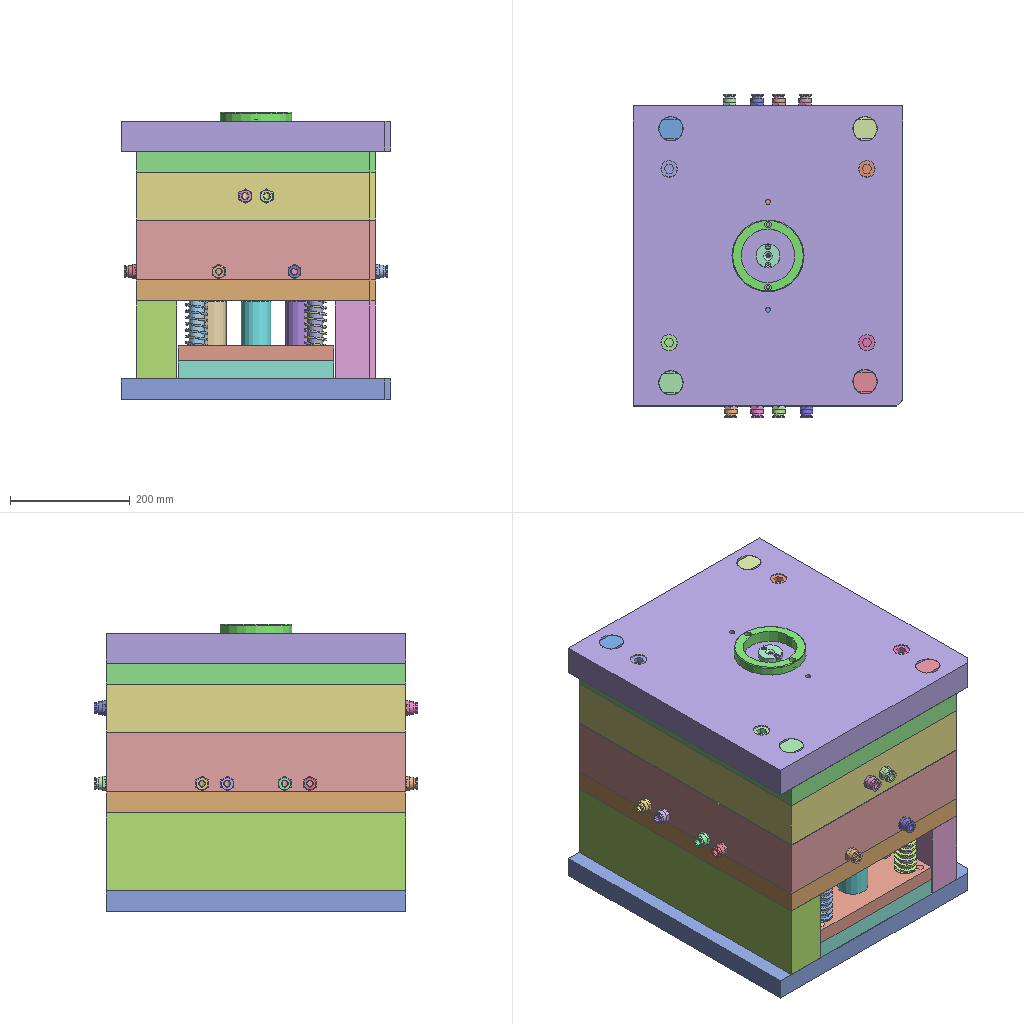Assembly | STEP file | 188 different items | 188 placed | box 450 x 540 x 480 mm
Parts list (item | name | quantity | parent item | size | volume):
1 | 1_id114_xmt_txt | x1 | in SL2-MOLD_xmt_txt | 21 x 31.9 x 24.249 mm | 5376 mm3
2 | 1_id118_xmt_txt | x1 | in SL2-MOLD_xmt_txt | 21 x 31.9 x 24.249 mm | 5376 mm3
3 | 1_id122_xmt_txt | x1 | in SL2-MOLD_xmt_txt | 21 x 31.9 x 24.249 mm | 5376 mm3
4 | 1_id126_xmt_txt | x1 | in SL2-MOLD_xmt_txt | 21 x 31.9 x 24.249 mm | 5376 mm3
5 | 1_id130_xmt_txt | x1 | in SL2-MOLD_xmt_txt | 10 x 10 x 26 mm | 960.822 mm3
6 | 1_id134_xmt_txt | x1 | in SL2-MOLD_xmt_txt | 10 x 10 x 26 mm | 960.822 mm3
7 | 1_id138_xmt_txt | x1 | in SL2-MOLD_xmt_txt | 10 x 10 x 26 mm | 960.822 mm3
8 | 1_id142_xmt_txt | x1 | in SL2-MOLD_xmt_txt | 10 x 10 x 26 mm | 960.822 mm3
9 | 1_id146_xmt_txt | x1 | in SL2-MOLD_xmt_txt | 10 x 10 x 26 mm | 960.822 mm3
10 | 1_id150_xmt_txt | x1 | in SL2-MOLD_xmt_txt | 10 x 10 x 26 mm | 960.822 mm3
11 | 1_id154_xmt_txt | x1 | in SL2-MOLD_xmt_txt | 10 x 10 x 26 mm | 960.822 mm3
12 | 1_id158_xmt_txt | x1 | in SL2-MOLD_xmt_txt | 10 x 10 x 26 mm | 960.822 mm3
13 | 1_id162_xmt_txt | x1 | in SL2-MOLD_xmt_txt | 10 x 10 x 26 mm | 960.822 mm3
14 | 1_id166_xmt_txt | x1 | in SL2-MOLD_xmt_txt | 10 x 10 x 26 mm | 960.822 mm3
15 | 1_id170_xmt_txt | x1 | in SL2-MOLD_xmt_txt | 10 x 10 x 26 mm | 960.822 mm3
16 | 1_id174_xmt_txt | x1 | in SL2-MOLD_xmt_txt | 10 x 10 x 26 mm | 960.822 mm3
17 | 1_id282_xmt_txt | x1 | in SL2-MOLD_xmt_txt | 21 x 31.9 x 24.249 mm | 5376 mm3
18 | 1_id286_xmt_txt | x1 | in SL2-MOLD_xmt_txt | 21 x 31.9 x 24.249 mm | 5376 mm3
19 | 1_id290_xmt_txt | x1 | in SL2-MOLD_xmt_txt | 21 x 31.9 x 24.249 mm | 5376 mm3
20 | 1_id294_xmt_txt | x1 | in SL2-MOLD_xmt_txt | 21 x 31.9 x 24.249 mm | 5376 mm3
21 | 1_id298_xmt_txt | x1 | in SL2-MOLD_xmt_txt | 31.9 x 21 x 24.249 mm | 5376 mm3
22 | 1_id302_xmt_txt | x1 | in SL2-MOLD_xmt_txt | 31.9 x 21 x 24.249 mm | 5376 mm3
23 | 1_id306_xmt_txt | x1 | in SL2-MOLD_xmt_txt | 31.9 x 21 x 24.249 mm | 5376 mm3
24 | 1_id310_xmt_txt | x1 | in SL2-MOLD_xmt_txt | 31.9 x 21 x 24.249 mm | 5376 mm3
25 | 1_id314_xmt_txt | x1 | in SL2-MOLD_xmt_txt | 31.9 x 21 x 24.249 mm | 5376 mm3
26 | 1_id318_xmt_txt | x1 | in SL2-MOLD_xmt_txt | 31.9 x 21 x 24.249 mm | 5376 mm3
27 | 1_id322_xmt_txt | x1 | in SL2-MOLD_xmt_txt | 31.9 x 21 x 24.249 mm | 5376 mm3
28 | 1_id326_xmt_txt | x1 | in SL2-MOLD_xmt_txt | 31.9 x 21 x 24.249 mm | 5376 mm3
29 | 1_id330_xmt_txt | x1 | in SL2-MOLD_xmt_txt | 18 x 18 x 47 mm | 6453 mm3
30 | 1_id334_xmt_txt | x1 | in SL2-MOLD_xmt_txt | 18 x 18 x 47 mm | 6453 mm3
31 | 1_id338_xmt_txt | x1 | in SL2-MOLD_xmt_txt | 18 x 18 x 47 mm | 6453 mm3
32 | 1_id342_xmt_txt | x1 | in SL2-MOLD_xmt_txt | 18 x 18 x 47 mm | 6453 mm3
33 | 1_id346_xmt_txt | x1 | in SL2-MOLD_xmt_txt | 18 x 18 x 47 mm | 6453 mm3
34 | 1_id350_xmt_txt | x1 | in SL2-MOLD_xmt_txt | 18 x 18 x 47 mm | 6453 mm3
35 | 1_id442_xmt_txt | x1 | in SL2-MOLD_xmt_txt | 40 x 40 x 350 mm | 322067 mm3
36 | 1_id446_xmt_txt | x1 | in SL2-MOLD_xmt_txt | 40 x 40 x 350 mm | 322067 mm3
37 | 1_id450_xmt_txt | x1 | in SL2-MOLD_xmt_txt | 40 x 40 x 350 mm | 322067 mm3
38 | 1_id454_xmt_txt | x1 | in SL2-MOLD_xmt_txt | 40 x 40 x 350 mm | 322067 mm3
39 | 1_id458_xmt_txt | x1 | in SL2-MOLD_xmt_txt | 48.005 x 48.005 x 35 mm | 28920 mm3
40 | 1_id462_xmt_txt | x1 | in SL2-MOLD_xmt_txt | 48.005 x 48.005 x 35 mm | 28920 mm3
41 | 1_id466_xmt_txt | x1 | in SL2-MOLD_xmt_txt | 48.005 x 48.005 x 35 mm | 28920 mm3
42 | 1_id470_xmt_txt | x1 | in SL2-MOLD_xmt_txt | 48.005 x 48.005 x 35 mm | 28920 mm3
43 | 1_id474_xmt_txt | x1 | in SL2-MOLD_xmt_txt | 54 x 54 x 80 mm | 71084 mm3
44 | 1_id478_xmt_txt | x1 | in SL2-MOLD_xmt_txt | 54 x 54 x 80 mm | 71084 mm3
45 | 1_id482_xmt_txt | x1 | in SL2-MOLD_xmt_txt | 54 x 54 x 80 mm | 71084 mm3
46 | 1_id486_xmt_txt | x1 | in SL2-MOLD_xmt_txt | 54 x 54 x 80 mm | 71084 mm3
47 | 1_id490_xmt_txt | x1 | in SL2-MOLD_xmt_txt | 54 x 54 x 80 mm | 71084 mm3
48 | 1_id494_xmt_txt | x1 | in SL2-MOLD_xmt_txt | 54 x 54 x 80 mm | 71084 mm3
49 | 1_id498_xmt_txt | x1 | in SL2-MOLD_xmt_txt | 54 x 54 x 80 mm | 71084 mm3
50 | 1_id502_xmt_txt | x1 | in SL2-MOLD_xmt_txt | 54 x 54 x 80 mm | 71084 mm3
51 | 1_id506_xmt_txt | x1 | in SL2-MOLD_xmt_txt | 120 x 120 x 20 mm | 95777 mm3
52 | 1_id530_xmt_txt | x1 | in SL2-MOLD_xmt_txt | 8 x 8 x 63 mm | 1811 mm3
53 | 1_id534_xmt_txt | x1 | in SL2-MOLD_xmt_txt | 8 x 8 x 63 mm | 1811 mm3
54 | 1_id538_xmt_txt | x1 | in SL2-MOLD_xmt_txt | 28 x 28 x 214 mm | 66281 mm3
55 | 1_id542_xmt_txt | x1 | in SL2-MOLD_xmt_txt | 28 x 28 x 214 mm | 66281 mm3
56 | 1_id546_xmt_txt | x1 | in SL2-MOLD_xmt_txt | 28 x 28 x 214 mm | 66281 mm3
57 | 1_id550_xmt_txt | x1 | in SL2-MOLD_xmt_txt | 28 x 28 x 214 mm | 66281 mm3
58 | 1_id554_xmt_txt | x1 | in SL2-MOLD_xmt_txt | 27 x 27 x 96 mm | 22322 mm3
59 | 1_id558_xmt_txt | x1 | in SL2-MOLD_xmt_txt | 27 x 27 x 96 mm | 22322 mm3
60 | 1_id562_xmt_txt | x1 | in SL2-MOLD_xmt_txt | 27 x 27 x 96 mm | 22322 mm3
61 | 1_id566_xmt_txt | x1 | in SL2-MOLD_xmt_txt | 27 x 27 x 96 mm | 22322 mm3
62 | 1_id570_xmt_txt | x1 | in SL2-MOLD_xmt_txt | 20 x 20 x 44 mm | 10770 mm3
63 | 1_id574_xmt_txt | x1 | in SL2-MOLD_xmt_txt | 20 x 20 x 44 mm | 10770 mm3
64 | 1_id578_xmt_txt | x1 | in SL2-MOLD_xmt_txt | 20 x 20 x 44 mm | 10770 mm3
65 | 1_id582_xmt_txt | x1 | in SL2-MOLD_xmt_txt | 20 x 20 x 44 mm | 10770 mm3
66 | 1_id586_xmt_txt | x1 | in SL2-MOLD_xmt_txt | 24 x 24 x 236 mm | 50039 mm3
67 | 1_id58_xmt_txt | x1 | in SL2-MOLD_xmt_txt | 18 x 18 x 47 mm | 6453 mm3
68 | 1_id590_xmt_txt | x1 | in SL2-MOLD_xmt_txt | 24 x 24 x 236 mm | 50039 mm3
69 | 1_id594_xmt_txt | x1 | in SL2-MOLD_xmt_txt | 24 x 24 x 236 mm | 50039 mm3
70 | 1_id598_xmt_txt | x1 | in SL2-MOLD_xmt_txt | 24 x 24 x 236 mm | 50039 mm3
71 | 1_id602_xmt_txt | x1 | in SL2-MOLD_xmt_txt | 24 x 24 x 236 mm | 50039 mm3
72 | 1_id606_xmt_txt | x1 | in SL2-MOLD_xmt_txt | 24 x 24 x 236 mm | 50039 mm3
73 | 1_id610_xmt_txt | x1 | in SL2-MOLD_xmt_txt | 18 x 18 x 55 mm | 7362 mm3
74 | 1_id614_xmt_txt | x1 | in SL2-MOLD_xmt_txt | 18 x 18 x 55 mm | 7362 mm3
75 | 1_id618_xmt_txt | x1 | in SL2-MOLD_xmt_txt | 18 x 18 x 55 mm | 7362 mm3
76 | 1_id622_xmt_txt | x1 | in SL2-MOLD_xmt_txt | 18 x 18 x 55 mm | 7362 mm3
77 | 1_id626_xmt_txt | x1 | in SL2-MOLD_xmt_txt | 18 x 18 x 55 mm | 7362 mm3
78 | 1_id62_xmt_txt | x1 | in SL2-MOLD_xmt_txt | 18 x 18 x 47 mm | 6453 mm3
79 | 1_id630_xmt_txt | x1 | in SL2-MOLD_xmt_txt | 18 x 18 x 55 mm | 7362 mm3
80 | 1_id634_xmt_txt | x1 | in SL2-MOLD_xmt_txt | 30 x 30 x 231 mm | 114179 mm3
81 | 1_id638_xmt_txt | x1 | in SL2-MOLD_xmt_txt | 30 x 30 x 231 mm | 114179 mm3
82 | 1_id642_xmt_txt | x1 | in SL2-MOLD_xmt_txt | 30 x 30 x 231 mm | 114179 mm3
83 | 1_id646_xmt_txt | x1 | in SL2-MOLD_xmt_txt | 30 x 30 x 231 mm | 114179 mm3
84 | 1_id654_xmt_txt | x1 | in SL2-MOLD_xmt_txt | 37 x 37 x 150 mm | 21369 mm3
85 | 1_id658_xmt_txt | x1 | in SL2-MOLD_xmt_txt | 37 x 37 x 150 mm | 21369 mm3
86 | 1_id662_xmt_txt | x1 | in SL2-MOLD_xmt_txt | 37 x 37 x 150 mm | 21369 mm3
87 | 1_id666_xmt_txt | x1 | in SL2-MOLD_xmt_txt | 37 x 37 x 150 mm | 21369 mm3
88 | 1_id66_xmt_txt | x1 | in SL2-MOLD_xmt_txt | 18 x 18 x 47 mm | 6453 mm3
89 | 1_id670_xmt_txt | x1 | in SL2-MOLD_xmt_txt | 28 x 28 x 185 mm | 57057 mm3
90 | 1_id674_xmt_txt | x1 | in SL2-MOLD_xmt_txt | 28 x 28 x 185 mm | 57057 mm3
91 | 1_id678_xmt_txt | x1 | in SL2-MOLD_xmt_txt | 28 x 28 x 185 mm | 57057 mm3
92 | 1_id682_xmt_txt | x1 | in SL2-MOLD_xmt_txt | 28 x 28 x 185 mm | 57057 mm3
93 | 1_id686_xmt_txt | x1 | in SL2-MOLD_xmt_txt | 18 x 18 x 47 mm | 6453 mm3
94 | 1_id690_xmt_txt | x1 | in SL2-MOLD_xmt_txt | 18 x 18 x 47 mm | 6453 mm3
95 | 1_id694_xmt_txt | x1 | in SL2-MOLD_xmt_txt | 18 x 18 x 47 mm | 6453 mm3
96 | 1_id698_xmt_txt | x1 | in SL2-MOLD_xmt_txt | 18 x 18 x 47 mm | 6453 mm3
97 | 1_id706_xmt_txt | x1 | in SL2-MOLD_xmt_txt | 40 x 40 x 95 mm | 34804 mm3
98 | 1_id70_xmt_txt | x1 | in SL2-MOLD_xmt_txt | 18 x 18 x 47 mm | 6453 mm3
99 | 1_id74_xmt_txt | x1 | in SL2-MOLD_xmt_txt | 18 x 18 x 47 mm | 6453 mm3
100 | 1_id78_xmt_txt | x1 | in SL2-MOLD_xmt_txt | 18 x 18 x 47 mm | 6453 mm3
101 | 1_id82_xmt_txt | x1 | in SL2-MOLD_xmt_txt | 18 x 18 x 47 mm | 6453 mm3
102 | 1_id86_xmt_txt | x1 | in SL2-MOLD_xmt_txt | 18 x 18 x 47 mm | 6453 mm3
103 | 2_id514_xmt_txt | x1 | in SL2-MOLD_xmt_txt | 8.5 x 8.5 x 17 mm | 477.285 mm3
104 | 3_id510_xmt_txt | x1 | in SL2-MOLD_xmt_txt | 8.5 x 8.5 x 17 mm | 477.285 mm3
105 | SL2-MOLD_id102_xmt_txt | x1 | in SL2-MOLD_xmt_txt | 50 x 50 x 130 mm | 253722 mm3
106 | SL2-MOLD_id106_xmt_txt | x1 | in SL2-MOLD_xmt_txt | 50 x 50 x 130 mm | 253722 mm3
107 | SL2-MOLD_id10_xmt_txt | x1 | in SL2-MOLD_xmt_txt | 50 x 11.99 x 16.246 mm | 7285 mm3
108 | SL2-MOLD_id110_xmt_txt | x1 | in SL2-MOLD_xmt_txt | 50 x 50 x 130 mm | 253722 mm3
109 | SL2-MOLD_id14_xmt_txt | x1 | in SL2-MOLD_xmt_txt | 45 x 110 x 10 mm | 48642 mm3
110 | SL2-MOLD_id178_xmt_txt | x1 | in SL2-MOLD_xmt_txt | 20 x 20 x 95 mm | 5358 mm3
111 | SL2-MOLD_id182_xmt_txt | x1 | in SL2-MOLD_xmt_txt | 20 x 20 x 95 mm | 5358 mm3
112 | SL2-MOLD_id186_xmt_txt | x1 | in SL2-MOLD_xmt_txt | 20 x 20 x 95 mm | 5358 mm3
113 | SL2-MOLD_id18_xmt_txt | x1 | in SL2-MOLD_xmt_txt | 110 x 40 x 10 mm | 43142 mm3
114 | SL2-MOLD_id190_xmt_txt | x1 | in SL2-MOLD_xmt_txt | 20 x 20 x 95 mm | 5358 mm3
115 | SL2-MOLD_id194_xmt_txt | x1 | in SL2-MOLD_xmt_txt | 20 x 20 x 95 mm | 5358 mm3
116 | SL2-MOLD_id198_xmt_txt | x1 | in SL2-MOLD_xmt_txt | 20 x 20 x 95 mm | 5358 mm3
117 | SL2-MOLD_id202_xmt_txt | x1 | in SL2-MOLD_xmt_txt | 20 x 20 x 95 mm | 5358 mm3
118 | SL2-MOLD_id206_xmt_txt | x1 | in SL2-MOLD_xmt_txt | 20 x 20 x 95 mm | 5358 mm3
119 | SL2-MOLD_id210_xmt_txt | x1 | in SL2-MOLD_xmt_txt | 20 x 20 x 95 mm | 5358 mm3
120 | SL2-MOLD_id214_xmt_txt | x1 | in SL2-MOLD_xmt_txt | 20 x 20 x 95 mm | 5358 mm3
121 | SL2-MOLD_id218_xmt_txt | x1 | in SL2-MOLD_xmt_txt | 20 x 20 x 95 mm | 5358 mm3
122 | SL2-MOLD_id222_xmt_txt | x1 | in SL2-MOLD_xmt_txt | 20 x 20 x 95 mm | 5358 mm3
123 | SL2-MOLD_id226_xmt_txt | x1 | in SL2-MOLD_xmt_txt | 20 x 20 x 95 mm | 5358 mm3
124 | SL2-MOLD_id22_xmt_txt | x1 | in SL2-MOLD_xmt_txt | 110 x 40 x 10 mm | 43142 mm3
125 | SL2-MOLD_id230_xmt_txt | x1 | in SL2-MOLD_xmt_txt | 20 x 20 x 95 mm | 5358 mm3
126 | SL2-MOLD_id234_xmt_txt | x1 | in SL2-MOLD_xmt_txt | 20 x 20 x 95 mm | 5358 mm3
127 | SL2-MOLD_id238_xmt_txt | x1 | in SL2-MOLD_xmt_txt | 20 x 20 x 95 mm | 5358 mm3
128 | SL2-MOLD_id242_xmt_txt | x1 | in SL2-MOLD_xmt_txt | 20 x 20 x 95 mm | 5358 mm3
129 | SL2-MOLD_id246_xmt_txt | x1 | in SL2-MOLD_xmt_txt | 20 x 20 x 95 mm | 5358 mm3
130 | SL2-MOLD_id250_xmt_txt | x1 | in SL2-MOLD_xmt_txt | 20 x 20 x 95 mm | 5358 mm3
131 | SL2-MOLD_id254_xmt_txt | x1 | in SL2-MOLD_xmt_txt | 20 x 20 x 95 mm | 5358 mm3
132 | SL2-MOLD_id258_xmt_txt | x1 | in SL2-MOLD_xmt_txt | 20 x 20 x 95 mm | 5358 mm3
133 | SL2-MOLD_id262_xmt_txt | x1 | in SL2-MOLD_xmt_txt | 20 x 20 x 95 mm | 5358 mm3
134 | SL2-MOLD_id266_xmt_txt | x1 | in SL2-MOLD_xmt_txt | 20 x 20 x 95 mm | 5358 mm3
135 | SL2-MOLD_id26_xmt_txt | x1 | in SL2-MOLD_xmt_txt | 45 x 110 x 10 mm | 48642 mm3
136 | SL2-MOLD_id270_xmt_txt | x1 | in SL2-MOLD_xmt_txt | 20 x 20 x 95 mm | 5358 mm3
137 | SL2-MOLD_id274_xmt_txt | x1 | in SL2-MOLD_xmt_txt | 20 x 20 x 95 mm | 5358 mm3
138 | SL2-MOLD_id278_xmt_txt | x1 | in SL2-MOLD_xmt_txt | 20 x 20 x 95 mm | 5358 mm3
139 | SL2-MOLD_id30_xmt_txt | x1 | in SL2-MOLD_xmt_txt | 11.99 x 50 x 16.246 mm | 7285 mm3
140 | SL2-MOLD_id34_xmt_txt | x1 | in SL2-MOLD_xmt_txt | 11.99 x 50 x 16.246 mm | 7285 mm3
141 | SL2-MOLD_id354_xmt_txt | x1 | in SL2-MOLD_xmt_txt | 265 x 420 x 8 mm | 688291 mm3
142 | SL2-MOLD_id358_xmt_txt | x1 | in SL2-MOLD_xmt_txt | 22 x 22 x 70 mm | 6058 mm3
143 | SL2-MOLD_id362_xmt_txt | x1 | in SL2-MOLD_xmt_txt | 22 x 22 x 70 mm | 6058 mm3
144 | SL2-MOLD_id366_xmt_txt | x1 | in SL2-MOLD_xmt_txt | 22 x 22 x 70 mm | 6058 mm3
145 | SL2-MOLD_id370_xmt_txt | x1 | in SL2-MOLD_xmt_txt | 22 x 22 x 70 mm | 6058 mm3
146 | SL2-MOLD_id374_xmt_txt | x1 | in SL2-MOLD_xmt_txt | 22 x 22 x 70 mm | 6058 mm3
147 | SL2-MOLD_id378_xmt_txt | x1 | in SL2-MOLD_xmt_txt | 22 x 22 x 70 mm | 6058 mm3
148 | SL2-MOLD_id382_xmt_txt | x1 | in SL2-MOLD_xmt_txt | 22 x 22 x 70 mm | 6058 mm3
149 | SL2-MOLD_id386_xmt_txt | x1 | in SL2-MOLD_xmt_txt | 22 x 22 x 70 mm | 6058 mm3
150 | SL2-MOLD_id38_xmt_txt | x1 | in SL2-MOLD_xmt_txt | 11.99 x 50 x 16.246 mm | 7285 mm3
151 | SL2-MOLD_id390_xmt_txt | x1 | in SL2-MOLD_xmt_txt | 22 x 22 x 70 mm | 6058 mm3
152 | SL2-MOLD_id394_xmt_txt | x1 | in SL2-MOLD_xmt_txt | 22 x 22 x 70 mm | 6058 mm3
153 | SL2-MOLD_id398_xmt_txt | x1 | in SL2-MOLD_xmt_txt | 22 x 22 x 70 mm | 6058 mm3
154 | SL2-MOLD_id402_xmt_txt | x1 | in SL2-MOLD_xmt_txt | 22 x 22 x 70 mm | 6058 mm3
155 | SL2-MOLD_id406_xmt_txt | x1 | in SL2-MOLD_xmt_txt | 22 x 22 x 70 mm | 6058 mm3
156 | SL2-MOLD_id410_xmt_txt | x1 | in SL2-MOLD_xmt_txt | 22 x 22 x 70 mm | 6058 mm3
157 | SL2-MOLD_id414_xmt_txt | x1 | in SL2-MOLD_xmt_txt | 22 x 22 x 70 mm | 6058 mm3
158 | SL2-MOLD_id418_xmt_txt | x1 | in SL2-MOLD_xmt_txt | 22 x 22 x 70 mm | 6058 mm3
159 | SL2-MOLD_id422_xmt_txt | x1 | in SL2-MOLD_xmt_txt | 22 x 22 x 70 mm | 6058 mm3
160 | SL2-MOLD_id426_xmt_txt | x1 | in SL2-MOLD_xmt_txt | 22 x 22 x 70 mm | 6058 mm3
161 | SL2-MOLD_id42_xmt_txt | x1 | in SL2-MOLD_xmt_txt | 11.99 x 50 x 16.246 mm | 7285 mm3
162 | SL2-MOLD_id430_xmt_txt | x1 | in SL2-MOLD_xmt_txt | 22 x 22 x 70 mm | 6058 mm3
163 | SL2-MOLD_id434_xmt_txt | x1 | in SL2-MOLD_xmt_txt | 22 x 22 x 70 mm | 6058 mm3
164 | SL2-MOLD_id438_xmt_txt | x1 | in SL2-MOLD_xmt_txt | 22 x 22 x 70 mm | 6058 mm3
165 | SL2-MOLD_id46_xmt_txt | x1 | in SL2-MOLD_xmt_txt | 11.99 x 50 x 16.246 mm | 7285 mm3
166 | SL2-MOLD_id50_xmt_txt | x1 | in SL2-MOLD_xmt_txt | 11.99 x 50 x 16.246 mm | 7285 mm3
167 | SL2-MOLD_id518_xmt_txt | x1 | in SL2-MOLD_xmt_txt | 5.668 x 5.668 x 36.992 mm | 436.735 mm3
168 | SL2-MOLD_id522_xmt_txt | x1 | in SL2-MOLD_xmt_txt | 5.668 x 5.668 x 36.992 mm | 436.735 mm3
169 | SL2-MOLD_id526_xmt_txt | x1 | in SL2-MOLD_xmt_txt | 50.634 x 195.983 x 4 mm | 4499 mm3
170 | SL2-MOLD_id54_xmt_txt | x1 | in SL2-MOLD_xmt_txt | 400 x 500 x 100 mm | 12901119 mm3
171 | SL2-MOLD_id650_xmt_txt | x1 | in SL2-MOLD_xmt_txt | 260 x 400 x 30 mm | 1707580 mm3
172 | SL2-MOLD_id6_xmt_txt | x1 | in SL2-MOLD_xmt_txt | 50 x 11.99 x 16.246 mm | 7285 mm3
173 | SL2-MOLD_id702_xmt_txt | x1 | in SL2-MOLD_xmt_txt | 260 x 500 x 25 mm | 2824522 mm3
174 | SL2-MOLD_id710_xmt_txt | x1 | in SL2-MOLD_xmt_txt | 177.394 x 134.722 x 72.136 mm | 76295 mm3
175 | SL2-MOLD_id714_xmt_txt | x1 | in SL2-MOLD_xmt_txt | 177.394 x 134.722 x 72.136 mm | 76295 mm3
176 | SL2-MOLD_id718_xmt_txt | x1 | in SL2-MOLD_xmt_txt | 172.262 x 129.59 x 111.89 mm | 1963711 mm3
177 | SL2-MOLD_id722_xmt_txt | x1 | in SL2-MOLD_xmt_txt | 172.262 x 129.59 x 111.89 mm | 1963711 mm3
178 | SL2-MOLD_id726_xmt_txt | x1 | in SL2-MOLD_xmt_txt | 400 x 500 x 35 mm | 6713866 mm3
179 | SL2-MOLD_id730_xmt_txt | x1 | in SL2-MOLD_xmt_txt | 450 x 500 x 50 mm | 10885298 mm3
180 | SL2-MOLD_id734_xmt_txt | x1 | in SL2-MOLD_xmt_txt | 400 x 500 x 35 mm | 6503504 mm3
181 | SL2-MOLD_id738_xmt_txt | x1 | in SL2-MOLD_xmt_txt | 260 x 500 x 30 mm | 3495338 mm3
182 | SL2-MOLD_id742_xmt_txt | x1 | in SL2-MOLD_xmt_txt | 68 x 500 x 130 mm | 4074828 mm3
183 | SL2-MOLD_id746_xmt_txt | x1 | in SL2-MOLD_xmt_txt | 68 x 500 x 130 mm | 4081328 mm3
184 | SL2-MOLD_id750_xmt_txt | x1 | in SL2-MOLD_xmt_txt | 450 x 500 x 35 mm | 7734159 mm3
185 | SL2-MOLD_id754_xmt_txt | x1 | in SL2-MOLD_xmt_txt | 400 x 500 x 99 mm | 12276978 mm3
186 | SL2-MOLD_id90_xmt_txt | x1 | in SL2-MOLD_xmt_txt | 50 x 50 x 130 mm | 253722 mm3
187 | SL2-MOLD_id94_xmt_txt | x1 | in SL2-MOLD_xmt_txt | 50 x 50 x 130 mm | 253722 mm3
188 | SL2-MOLD_id98_xmt_txt | x1 | in SL2-MOLD_xmt_txt | 50 x 50 x 130 mm | 253722 mm3